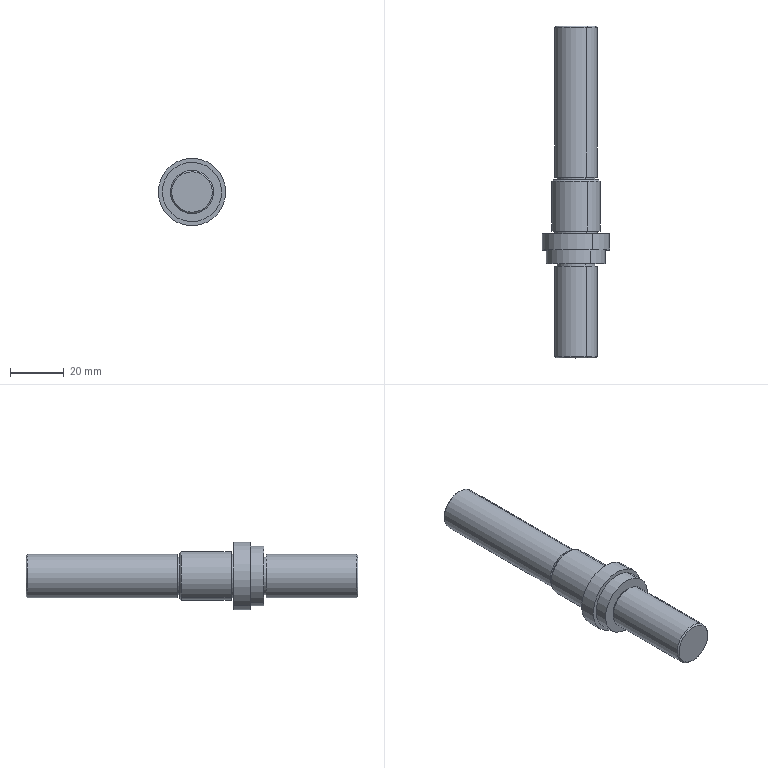Part | STEP file | 20304 | 1 solid | 31 faces | box 25 x 123 x 25 mm | volume 28266 mm3 | cylinder 16 | plane 9 | cone 6 | commonest cylinder face diameters 16 x6 14 x4 18 x2 22 x2 25 x2
STEP:
#1=CARTESIAN_POINT('',(3.356,-56.,6.143));
#2=VERTEX_POINT('',#1);
#3=CARTESIAN_POINT('',(-3.356,-56.,-6.143));
#4=VERTEX_POINT('',#3);
#5=CARTESIAN_POINT('',(0.,-56.,0.));
#6=DIRECTION('',(0.,1.,0.));
#7=AXIS2_PLACEMENT_3D('',#5,#6,$);
#8=CIRCLE('',#7,7.);
#9=EDGE_CURVE('',#2,#4,#8,.T.);
#10=ORIENTED_EDGE('',*,*,#9,.F.);
#11=CARTESIAN_POINT('',(3.356,-57.,6.143));
#12=VERTEX_POINT('',#11);
#13=CARTESIAN_POINT('',(3.356,-72.5,6.143));
#14=DIRECTION('',(0.,1.,0.));
#15=VECTOR('',#14,1.);
#16=LINE('',#13,#15);
#17=EDGE_CURVE('',#2,#12,#16,.F.);
#18=ORIENTED_EDGE('',*,*,#17,.T.);
#19=CARTESIAN_POINT('',(-3.356,-57.,-6.143));
#20=VERTEX_POINT('',#19);
#21=CARTESIAN_POINT('',(0.,-57.,0.));
#22=DIRECTION('',(0.,1.,0.));
#23=AXIS2_PLACEMENT_3D('',#21,#22,$);
#24=CIRCLE('',#23,7.);
#25=EDGE_CURVE('',#12,#20,#24,.T.);
#26=ORIENTED_EDGE('',*,*,#25,.T.);
#27=CARTESIAN_POINT('',(-3.356,-72.5,-6.143));
#28=DIRECTION('',(0.,1.,0.));
#29=VECTOR('',#28,1.);
#30=LINE('',#27,#29);
#31=EDGE_CURVE('',#4,#20,#30,.F.);
#32=ORIENTED_EDGE('',*,*,#31,.F.);
#33=EDGE_LOOP('',(#10,#18,#26,#32));
#34=FACE_OUTER_BOUND('',#33,.T.);
#35=CARTESIAN_POINT('',(0.,-61.5,0.));
#36=DIRECTION('',(0.,1.,0.));
#37=DIRECTION('',(0.4794,0.,0.8776));
#38=AXIS2_PLACEMENT_3D('',#35,#36,#37);
#39=CYLINDRICAL_SURFACE('',#38,7.);
#40=ADVANCED_FACE('',(#34),#39,.T.);
#41=CARTESIAN_POINT('',(0.,-56.,0.));
#42=DIRECTION('',(0.,1.,0.));
#43=AXIS2_PLACEMENT_3D('',#41,#42,$);
#44=CIRCLE('',#43,7.);
#45=EDGE_CURVE('',#4,#2,#44,.T.);
#46=ORIENTED_EDGE('',*,*,#45,.F.);
#47=ORIENTED_EDGE('',*,*,#31,.T.);
#48=CARTESIAN_POINT('',(0.,-57.,0.));
#49=DIRECTION('',(0.,1.,0.));
#50=AXIS2_PLACEMENT_3D('',#48,#49,$);
#51=CIRCLE('',#50,7.);
#52=EDGE_CURVE('',#20,#12,#51,.T.);
#53=ORIENTED_EDGE('',*,*,#52,.T.);
#54=ORIENTED_EDGE('',*,*,#17,.F.);
#55=EDGE_LOOP('',(#46,#47,#53,#54));
#56=FACE_OUTER_BOUND('',#55,.T.);
#57=ADVANCED_FACE('',(#56),#39,.T.);
#58=CARTESIAN_POINT('',(3.835,-76.,7.021));
#59=VERTEX_POINT('',#58);
#60=CARTESIAN_POINT('',(-3.835,-76.,-7.021));
#61=VERTEX_POINT('',#60);
#62=CARTESIAN_POINT('',(0.,-76.,0.));
#63=DIRECTION('',(0.,1.,0.));
#64=AXIS2_PLACEMENT_3D('',#62,#63,$);
#65=CIRCLE('',#64,8.);
#66=EDGE_CURVE('',#59,#61,#65,.T.);
#67=ORIENTED_EDGE('',*,*,#66,.F.);
#68=CARTESIAN_POINT('',(3.835,-77.,7.021));
#69=VERTEX_POINT('',#68);
#70=CARTESIAN_POINT('',(3.835,-61.5,7.021));
#71=DIRECTION('',(0.,1.,0.));
#72=VECTOR('',#71,1.);
#73=LINE('',#70,#72);
#74=EDGE_CURVE('',#59,#69,#73,.F.);
#75=ORIENTED_EDGE('',*,*,#74,.T.);
#76=CARTESIAN_POINT('',(-3.835,-77.,-7.021));
#77=VERTEX_POINT('',#76);
#78=CARTESIAN_POINT('',(0.,-77.,0.));
#79=DIRECTION('',(0.,1.,0.));
#80=AXIS2_PLACEMENT_3D('',#78,#79,$);
#81=CIRCLE('',#80,8.);
#82=EDGE_CURVE('',#69,#77,#81,.T.);
#83=ORIENTED_EDGE('',*,*,#82,.T.);
#84=CARTESIAN_POINT('',(-3.835,-61.5,-7.021));
#85=DIRECTION('',(0.,1.,0.));
#86=VECTOR('',#85,1.);
#87=LINE('',#84,#86);
#88=EDGE_CURVE('',#61,#77,#87,.F.);
#89=ORIENTED_EDGE('',*,*,#88,.F.);
#90=EDGE_LOOP('',(#67,#75,#83,#89));
#91=FACE_OUTER_BOUND('',#90,.T.);
#92=CARTESIAN_POINT('',(0.,-61.5,0.));
#93=DIRECTION('',(0.,1.,0.));
#94=DIRECTION('',(0.4794,0.,0.8776));
#95=AXIS2_PLACEMENT_3D('',#92,#93,#94);
#96=CYLINDRICAL_SURFACE('',#95,8.);
#97=ADVANCED_FACE('',(#91),#96,.T.);
#98=CARTESIAN_POINT('',(0.,-76.,0.));
#99=DIRECTION('',(0.,1.,0.));
#100=AXIS2_PLACEMENT_3D('',#98,#99,$);
#101=CIRCLE('',#100,8.);
#102=EDGE_CURVE('',#61,#59,#101,.T.);
#103=ORIENTED_EDGE('',*,*,#102,.F.);
#104=ORIENTED_EDGE('',*,*,#88,.T.);
#105=CARTESIAN_POINT('',(0.,-77.,0.));
#106=DIRECTION('',(0.,1.,0.));
#107=AXIS2_PLACEMENT_3D('',#105,#106,$);
#108=CIRCLE('',#107,8.);
#109=EDGE_CURVE('',#77,#69,#108,.T.);
#110=ORIENTED_EDGE('',*,*,#109,.T.);
#111=ORIENTED_EDGE('',*,*,#74,.F.);
#112=EDGE_LOOP('',(#103,#104,#110,#111));
#113=FACE_OUTER_BOUND('',#112,.T.);
#114=ADVANCED_FACE('',(#113),#96,.T.);
#115=CARTESIAN_POINT('',(5.993,-77.,10.97));
#116=VERTEX_POINT('',#115);
#117=CARTESIAN_POINT('',(-5.993,-77.,-10.97));
#118=VERTEX_POINT('',#117);
#119=CARTESIAN_POINT('',(0.,-77.,0.));
#120=DIRECTION('',(0.,1.,0.));
#121=AXIS2_PLACEMENT_3D('',#119,#120,$);
#122=CIRCLE('',#121,12.5);
#123=EDGE_CURVE('',#116,#118,#122,.T.);
#124=ORIENTED_EDGE('',*,*,#123,.F.);
#125=CARTESIAN_POINT('',(5.993,-83.,10.97));
#126=VERTEX_POINT('',#125);
#127=CARTESIAN_POINT('',(5.993,-80.,10.97));
#128=DIRECTION('',(0.,1.,0.));
#129=VECTOR('',#128,1.);
#130=LINE('',#127,#129);
#131=EDGE_CURVE('',#116,#126,#130,.F.);
#132=ORIENTED_EDGE('',*,*,#131,.T.);
#133=CARTESIAN_POINT('',(-5.993,-83.,-10.97));
#134=VERTEX_POINT('',#133);
#135=CARTESIAN_POINT('',(0.,-83.,0.));
#136=DIRECTION('',(0.,1.,0.));
#137=AXIS2_PLACEMENT_3D('',#135,#136,$);
#138=CIRCLE('',#137,12.5);
#139=EDGE_CURVE('',#126,#134,#138,.T.);
#140=ORIENTED_EDGE('',*,*,#139,.T.);
#141=CARTESIAN_POINT('',(-5.993,-80.,-10.97));
#142=DIRECTION('',(0.,1.,0.));
#143=VECTOR('',#142,1.);
#144=LINE('',#141,#143);
#145=EDGE_CURVE('',#118,#134,#144,.F.);
#146=ORIENTED_EDGE('',*,*,#145,.F.);
#147=EDGE_LOOP('',(#124,#132,#140,#146));
#148=FACE_OUTER_BOUND('',#147,.T.);
#149=CARTESIAN_POINT('',(0.,-61.5,0.));
#150=DIRECTION('',(0.,1.,0.));
#151=DIRECTION('',(0.4794,0.,0.8776));
#152=AXIS2_PLACEMENT_3D('',#149,#150,#151);
#153=CYLINDRICAL_SURFACE('',#152,12.5);
#154=ADVANCED_FACE('',(#148),#153,.T.);
#155=CARTESIAN_POINT('',(0.,-77.,0.));
#156=DIRECTION('',(0.,1.,0.));
#157=AXIS2_PLACEMENT_3D('',#155,#156,$);
#158=CIRCLE('',#157,12.5);
#159=EDGE_CURVE('',#118,#116,#158,.T.);
#160=ORIENTED_EDGE('',*,*,#159,.F.);
#161=ORIENTED_EDGE('',*,*,#145,.T.);
#162=CARTESIAN_POINT('',(0.,-83.,0.));
#163=DIRECTION('',(0.,1.,0.));
#164=AXIS2_PLACEMENT_3D('',#162,#163,$);
#165=CIRCLE('',#164,12.5);
#166=EDGE_CURVE('',#134,#126,#165,.T.);
#167=ORIENTED_EDGE('',*,*,#166,.T.);
#168=ORIENTED_EDGE('',*,*,#131,.F.);
#169=EDGE_LOOP('',(#160,#161,#167,#168));
#170=FACE_OUTER_BOUND('',#169,.T.);
#171=ADVANCED_FACE('',(#170),#153,.T.);
#172=CARTESIAN_POINT('',(5.274,-83.,9.653));
#173=VERTEX_POINT('',#172);
#174=CARTESIAN_POINT('',(-5.274,-83.,-9.653));
#175=VERTEX_POINT('',#174);
#176=CARTESIAN_POINT('',(0.,-83.,0.));
#177=DIRECTION('',(0.,1.,0.));
#178=AXIS2_PLACEMENT_3D('',#176,#177,$);
#179=CIRCLE('',#178,11.);
#180=EDGE_CURVE('',#173,#175,#179,.T.);
#181=ORIENTED_EDGE('',*,*,#180,.F.);
#182=CARTESIAN_POINT('',(5.274,-88.,9.653));
#183=VERTEX_POINT('',#182);
#184=CARTESIAN_POINT('',(5.274,-85.5,9.653));
#185=DIRECTION('',(0.,1.,0.));
#186=VECTOR('',#185,1.);
#187=LINE('',#184,#186);
#188=EDGE_CURVE('',#173,#183,#187,.F.);
#189=ORIENTED_EDGE('',*,*,#188,.T.);
#190=CARTESIAN_POINT('',(-5.274,-88.,-9.653));
#191=VERTEX_POINT('',#190);
#192=CARTESIAN_POINT('',(0.,-88.,0.));
#193=DIRECTION('',(0.,1.,0.));
#194=AXIS2_PLACEMENT_3D('',#192,#193,$);
#195=CIRCLE('',#194,11.);
#196=EDGE_CURVE('',#183,#191,#195,.T.);
#197=ORIENTED_EDGE('',*,*,#196,.T.);
#198=CARTESIAN_POINT('',(-5.274,-85.5,-9.653));
#199=DIRECTION('',(0.,1.,0.));
#200=VECTOR('',#199,1.);
#201=LINE('',#198,#200);
#202=EDGE_CURVE('',#175,#191,#201,.F.);
#203=ORIENTED_EDGE('',*,*,#202,.F.);
#204=EDGE_LOOP('',(#181,#189,#197,#203));
#205=FACE_OUTER_BOUND('',#204,.T.);
#206=CARTESIAN_POINT('',(0.,-61.5,0.));
#207=DIRECTION('',(0.,1.,0.));
#208=DIRECTION('',(0.4794,0.,0.8776));
#209=AXIS2_PLACEMENT_3D('',#206,#207,#208);
#210=CYLINDRICAL_SURFACE('',#209,11.);
#211=ADVANCED_FACE('',(#205),#210,.T.);
#212=CARTESIAN_POINT('',(0.,-83.,0.));
#213=DIRECTION('',(0.,1.,0.));
#214=AXIS2_PLACEMENT_3D('',#212,#213,$);
#215=CIRCLE('',#214,11.);
#216=EDGE_CURVE('',#175,#173,#215,.T.);
#217=ORIENTED_EDGE('',*,*,#216,.F.);
#218=ORIENTED_EDGE('',*,*,#202,.T.);
#219=CARTESIAN_POINT('',(0.,-88.,0.));
#220=DIRECTION('',(0.,1.,0.));
#221=AXIS2_PLACEMENT_3D('',#219,#220,$);
#222=CIRCLE('',#221,11.);
#223=EDGE_CURVE('',#191,#183,#222,.T.);
#224=ORIENTED_EDGE('',*,*,#223,.T.);
#225=ORIENTED_EDGE('',*,*,#188,.F.);
#226=EDGE_LOOP('',(#217,#218,#224,#225));
#227=FACE_OUTER_BOUND('',#226,.T.);
#228=ADVANCED_FACE('',(#227),#210,.T.);
#229=CARTESIAN_POINT('',(3.356,-88.,6.143));
#230=VERTEX_POINT('',#229);
#231=CARTESIAN_POINT('',(-3.356,-88.,-6.143));
#232=VERTEX_POINT('',#231);
#233=CARTESIAN_POINT('',(0.,-88.,0.));
#234=DIRECTION('',(0.,1.,0.));
#235=AXIS2_PLACEMENT_3D('',#233,#234,$);
#236=CIRCLE('',#235,7.);
#237=EDGE_CURVE('',#230,#232,#236,.T.);
#238=ORIENTED_EDGE('',*,*,#237,.F.);
#239=CARTESIAN_POINT('',(3.356,-89.,6.143));
#240=VERTEX_POINT('',#239);
#241=CARTESIAN_POINT('',(3.356,-72.5,6.143));
#242=DIRECTION('',(0.,1.,0.));
#243=VECTOR('',#242,1.);
#244=LINE('',#241,#243);
#245=EDGE_CURVE('',#230,#240,#244,.F.);
#246=ORIENTED_EDGE('',*,*,#245,.T.);
#247=CARTESIAN_POINT('',(-3.356,-89.,-6.143));
#248=VERTEX_POINT('',#247);
#249=CARTESIAN_POINT('',(0.,-89.,0.));
#250=DIRECTION('',(0.,1.,0.));
#251=AXIS2_PLACEMENT_3D('',#249,#250,$);
#252=CIRCLE('',#251,7.);
#253=EDGE_CURVE('',#240,#248,#252,.T.);
#254=ORIENTED_EDGE('',*,*,#253,.T.);
#255=CARTESIAN_POINT('',(-3.356,-72.5,-6.143));
#256=DIRECTION('',(0.,1.,0.));
#257=VECTOR('',#256,1.);
#258=LINE('',#255,#257);
#259=EDGE_CURVE('',#232,#248,#258,.F.);
#260=ORIENTED_EDGE('',*,*,#259,.F.);
#261=EDGE_LOOP('',(#238,#246,#254,#260));
#262=FACE_OUTER_BOUND('',#261,.T.);
#263=ADVANCED_FACE('',(#262),#39,.T.);
#264=CARTESIAN_POINT('',(0.,-88.,0.));
#265=DIRECTION('',(0.,1.,0.));
#266=AXIS2_PLACEMENT_3D('',#264,#265,$);
#267=CIRCLE('',#266,7.);
#268=EDGE_CURVE('',#232,#230,#267,.T.);
#269=ORIENTED_EDGE('',*,*,#268,.F.);
#270=ORIENTED_EDGE('',*,*,#259,.T.);
#271=CARTESIAN_POINT('',(0.,-89.,0.));
#272=DIRECTION('',(0.,1.,0.));
#273=AXIS2_PLACEMENT_3D('',#271,#272,$);
#274=CIRCLE('',#273,7.);
#275=EDGE_CURVE('',#248,#240,#274,.T.);
#276=ORIENTED_EDGE('',*,*,#275,.T.);
#277=ORIENTED_EDGE('',*,*,#245,.F.);
#278=EDGE_LOOP('',(#269,#270,#276,#277));
#279=FACE_OUTER_BOUND('',#278,.T.);
#280=ADVANCED_FACE('',(#279),#39,.T.);
#281=CARTESIAN_POINT('',(3.835,-56.,7.021));
#282=VERTEX_POINT('',#281);
#283=CARTESIAN_POINT('',(-3.835,-56.,-7.021));
#284=VERTEX_POINT('',#283);
#285=CARTESIAN_POINT('',(0.,-56.,0.));
#286=DIRECTION('',(0.,1.,0.));
#287=AXIS2_PLACEMENT_3D('',#285,#286,$);
#288=CIRCLE('',#287,8.);
#289=EDGE_CURVE('',#282,#284,#288,.T.);
#290=ORIENTED_EDGE('',*,*,#289,.F.);
#291=CARTESIAN_POINT('',(0.,-56.,0.));
#292=DIRECTION('',(0.,1.,0.));
#293=AXIS2_PLACEMENT_3D('',#291,#292,$);
#294=CIRCLE('',#293,8.);
#295=EDGE_CURVE('',#284,#282,#294,.T.);
#296=ORIENTED_EDGE('',*,*,#295,.F.);
#297=EDGE_LOOP('',(#290,#296));
#298=FACE_OUTER_BOUND('',#297,.T.);
#299=ORIENTED_EDGE('',*,*,#45,.T.);
#300=ORIENTED_EDGE('',*,*,#9,.T.);
#301=EDGE_LOOP('',(#299,#300));
#302=FACE_BOUND('',#301,.T.);
#303=CARTESIAN_POINT('',(0.,-56.,8.));
#304=DIRECTION('',(0.,1.,0.));
#305=DIRECTION('',(1.,0.,0.));
#306=AXIS2_PLACEMENT_3D('',#303,#304,#305);
#307=PLANE('',#306);
#308=ADVANCED_FACE('',(#298,#302),#307,.F.);
#309=CARTESIAN_POINT('',(4.315,-76.,7.898));
#310=VERTEX_POINT('',#309);
#311=CARTESIAN_POINT('',(-4.315,-76.,-7.898));
#312=VERTEX_POINT('',#311);
#313=CARTESIAN_POINT('',(0.,-76.,0.));
#314=DIRECTION('',(0.,1.,0.));
#315=AXIS2_PLACEMENT_3D('',#313,#314,$);
#316=CIRCLE('',#315,9.);
#317=EDGE_CURVE('',#310,#312,#316,.T.);
#318=ORIENTED_EDGE('',*,*,#317,.F.);
#319=CARTESIAN_POINT('',(0.,-76.,0.));
#320=DIRECTION('',(0.,1.,0.));
#321=AXIS2_PLACEMENT_3D('',#319,#320,$);
#322=CIRCLE('',#321,9.);
#323=EDGE_CURVE('',#312,#310,#322,.T.);
#324=ORIENTED_EDGE('',*,*,#323,.F.);
#325=EDGE_LOOP('',(#318,#324));
#326=FACE_OUTER_BOUND('',#325,.T.);
#327=ORIENTED_EDGE('',*,*,#102,.T.);
#328=ORIENTED_EDGE('',*,*,#66,.T.);
#329=EDGE_LOOP('',(#327,#328));
#330=FACE_BOUND('',#329,.T.);
#331=CARTESIAN_POINT('',(0.,-76.,9.));
#332=DIRECTION('',(0.,1.,0.));
#333=DIRECTION('',(1.,0.,0.));
#334=AXIS2_PLACEMENT_3D('',#331,#332,#333);
#335=PLANE('',#334);
#336=ADVANCED_FACE('',(#326,#330),#335,.F.);
#337=ORIENTED_EDGE('',*,*,#159,.T.);
#338=ORIENTED_EDGE('',*,*,#123,.T.);
#339=EDGE_LOOP('',(#337,#338));
#340=FACE_OUTER_BOUND('',#339,.T.);
#341=ORIENTED_EDGE('',*,*,#82,.F.);
#342=ORIENTED_EDGE('',*,*,#109,.F.);
#343=EDGE_LOOP('',(#341,#342));
#344=FACE_BOUND('',#343,.T.);
#345=CARTESIAN_POINT('',(0.,-77.,8.));
#346=DIRECTION('',(0.,1.,0.));
#347=DIRECTION('',(1.,0.,0.));
#348=AXIS2_PLACEMENT_3D('',#345,#346,#347);
#349=PLANE('',#348);
#350=ADVANCED_FACE('',(#340,#344),#349,.T.);
#351=ORIENTED_EDGE('',*,*,#139,.F.);
#352=ORIENTED_EDGE('',*,*,#166,.F.);
#353=EDGE_LOOP('',(#351,#352));
#354=FACE_OUTER_BOUND('',#353,.T.);
#355=ORIENTED_EDGE('',*,*,#216,.T.);
#356=ORIENTED_EDGE('',*,*,#180,.T.);
#357=EDGE_LOOP('',(#355,#356));
#358=FACE_BOUND('',#357,.T.);
#359=CARTESIAN_POINT('',(0.,-83.,12.5));
#360=DIRECTION('',(0.,1.,0.));
#361=DIRECTION('',(1.,0.,0.));
#362=AXIS2_PLACEMENT_3D('',#359,#360,#361);
#363=PLANE('',#362);
#364=ADVANCED_FACE('',(#354,#358),#363,.F.);
#365=ORIENTED_EDGE('',*,*,#196,.F.);
#366=ORIENTED_EDGE('',*,*,#223,.F.);
#367=EDGE_LOOP('',(#365,#366));
#368=FACE_OUTER_BOUND('',#367,.T.);
#369=ORIENTED_EDGE('',*,*,#268,.T.);
#370=ORIENTED_EDGE('',*,*,#237,.T.);
#371=EDGE_LOOP('',(#369,#370));
#372=FACE_BOUND('',#371,.T.);
#373=CARTESIAN_POINT('',(0.,-88.,11.));
#374=DIRECTION('',(0.,1.,0.));
#375=DIRECTION('',(1.,0.,0.));
#376=AXIS2_PLACEMENT_3D('',#373,#374,#375);
#377=PLANE('',#376);
#378=ADVANCED_FACE('',(#368,#372),#377,.F.);
#379=CARTESIAN_POINT('',(-3.835,-89.,-7.021));
#380=VERTEX_POINT('',#379);
#381=CARTESIAN_POINT('',(3.835,-89.,7.021));
#382=VERTEX_POINT('',#381);
#383=CARTESIAN_POINT('',(0.,-89.,0.));
#384=DIRECTION('',(0.,1.,0.));
#385=AXIS2_PLACEMENT_3D('',#383,#384,$);
#386=CIRCLE('',#385,8.);
#387=EDGE_CURVE('',#380,#382,#386,.T.);
#388=ORIENTED_EDGE('',*,*,#387,.T.);
#389=CARTESIAN_POINT('',(0.,-89.,0.));
#390=DIRECTION('',(0.,1.,0.));
#391=AXIS2_PLACEMENT_3D('',#389,#390,$);
#392=CIRCLE('',#391,8.);
#393=EDGE_CURVE('',#382,#380,#392,.T.);
#394=ORIENTED_EDGE('',*,*,#393,.T.);
#395=EDGE_LOOP('',(#388,#394));
#396=FACE_OUTER_BOUND('',#395,.T.);
#397=ORIENTED_EDGE('',*,*,#253,.F.);
#398=ORIENTED_EDGE('',*,*,#275,.F.);
#399=EDGE_LOOP('',(#397,#398));
#400=FACE_BOUND('',#399,.T.);
#401=CARTESIAN_POINT('',(0.,-89.,7.));
#402=DIRECTION('',(0.,1.,0.));
#403=DIRECTION('',(1.,0.,0.));
#404=AXIS2_PLACEMENT_3D('',#401,#402,#403);
#405=PLANE('',#404);
#406=ADVANCED_FACE('',(#396,#400),#405,.T.);
#407=CARTESIAN_POINT('',(3.835,-0.5,7.021));
#408=VERTEX_POINT('',#407);
#409=CARTESIAN_POINT('',(3.835,-61.5,7.021));
#410=DIRECTION('',(0.,1.,0.));
#411=VECTOR('',#410,1.);
#412=LINE('',#409,#411);
#413=EDGE_CURVE('',#408,#282,#412,.F.);
#414=ORIENTED_EDGE('',*,*,#413,.T.);
#415=ORIENTED_EDGE('',*,*,#289,.T.);
#416=CARTESIAN_POINT('',(-3.835,-0.5,-7.021));
#417=VERTEX_POINT('',#416);
#418=CARTESIAN_POINT('',(-3.835,-61.5,-7.021));
#419=DIRECTION('',(0.,1.,0.));
#420=VECTOR('',#419,1.);
#421=LINE('',#418,#420);
#422=EDGE_CURVE('',#417,#284,#421,.F.);
#423=ORIENTED_EDGE('',*,*,#422,.F.);
#424=CARTESIAN_POINT('',(0.,-0.5,0.));
#425=DIRECTION('',(0.,1.,0.));
#426=AXIS2_PLACEMENT_3D('',#424,#425,$);
#427=CIRCLE('',#426,8.);
#428=EDGE_CURVE('',#408,#417,#427,.T.);
#429=ORIENTED_EDGE('',*,*,#428,.F.);
#430=EDGE_LOOP('',(#414,#415,#423,#429));
#431=FACE_OUTER_BOUND('',#430,.T.);
#432=ADVANCED_FACE('',(#431),#96,.T.);
#433=ORIENTED_EDGE('',*,*,#422,.T.);
#434=ORIENTED_EDGE('',*,*,#295,.T.);
#435=ORIENTED_EDGE('',*,*,#413,.F.);
#436=CARTESIAN_POINT('',(0.,-0.5,0.));
#437=DIRECTION('',(0.,1.,0.));
#438=AXIS2_PLACEMENT_3D('',#436,#437,$);
#439=CIRCLE('',#438,8.);
#440=EDGE_CURVE('',#417,#408,#439,.T.);
#441=ORIENTED_EDGE('',*,*,#440,.F.);
#442=EDGE_LOOP('',(#433,#434,#435,#441));
#443=FACE_OUTER_BOUND('',#442,.T.);
#444=ADVANCED_FACE('',(#443),#96,.T.);
#445=CARTESIAN_POINT('',(3.596,0.,6.582));
#446=VERTEX_POINT('',#445);
#447=CARTESIAN_POINT('',(-3.596,0.,-6.582));
#448=VERTEX_POINT('',#447);
#449=CARTESIAN_POINT('',(0.,0.,0.));
#450=DIRECTION('',(0.,1.,0.));
#451=AXIS2_PLACEMENT_3D('',#449,#450,$);
#452=CIRCLE('',#451,7.5);
#453=EDGE_CURVE('',#446,#448,#452,.T.);
#454=ORIENTED_EDGE('',*,*,#453,.T.);
#455=CARTESIAN_POINT('',(0.,0.,0.));
#456=DIRECTION('',(0.,1.,0.));
#457=AXIS2_PLACEMENT_3D('',#455,#456,$);
#458=CIRCLE('',#457,7.5);
#459=EDGE_CURVE('',#448,#446,#458,.T.);
#460=ORIENTED_EDGE('',*,*,#459,.T.);
#461=EDGE_LOOP('',(#454,#460));
#462=FACE_OUTER_BOUND('',#461,.T.);
#463=CARTESIAN_POINT('',(0.,0.,0.));
#464=DIRECTION('',(0.,1.,0.));
#465=DIRECTION('',(1.,0.,0.));
#466=AXIS2_PLACEMENT_3D('',#463,#464,#465);
#467=PLANE('',#466);
#468=ADVANCED_FACE('',(#462),#467,.T.);
#469=CARTESIAN_POINT('',(3.716,-0.25,6.801));
#470=DIRECTION('',(0.339,-0.7071,0.6205));
#471=VECTOR('',#470,1.);
#472=LINE('',#469,#471);
#473=EDGE_CURVE('',#446,#408,#472,.T.);
#474=ORIENTED_EDGE('',*,*,#473,.T.);
#475=ORIENTED_EDGE('',*,*,#428,.T.);
#476=CARTESIAN_POINT('',(-3.716,-0.25,-6.801));
#477=DIRECTION('',(-0.339,-0.7071,-0.6205));
#478=VECTOR('',#477,1.);
#479=LINE('',#476,#478);
#480=EDGE_CURVE('',#448,#417,#479,.T.);
#481=ORIENTED_EDGE('',*,*,#480,.F.);
#482=ORIENTED_EDGE('',*,*,#453,.F.);
#483=EDGE_LOOP('',(#474,#475,#481,#482));
#484=FACE_OUTER_BOUND('',#483,.T.);
#485=CARTESIAN_POINT('',(0.,7.5,0.));
#486=DIRECTION('',(0.,-1.,0.));
#487=DIRECTION('',(0.4794,0.,0.8776));
#488=AXIS2_PLACEMENT_3D('',#485,#486,#487);
#489=CONICAL_SURFACE('',#488,0.,0.7854);
#490=ADVANCED_FACE('',(#484),#489,.T.);
#491=ORIENTED_EDGE('',*,*,#480,.T.);
#492=ORIENTED_EDGE('',*,*,#440,.T.);
#493=ORIENTED_EDGE('',*,*,#473,.F.);
#494=ORIENTED_EDGE('',*,*,#459,.F.);
#495=EDGE_LOOP('',(#491,#492,#493,#494));
#496=FACE_OUTER_BOUND('',#495,.T.);
#497=CARTESIAN_POINT('',(0.,7.5,0.));
#498=DIRECTION('',(0.,-1.,0.));
#499=DIRECTION('',(0.008915,0.,-1.));
#500=AXIS2_PLACEMENT_3D('',#497,#498,#499);
#501=CONICAL_SURFACE('',#500,0.,0.7854);
#502=ADVANCED_FACE('',(#496),#501,.T.);
#503=CARTESIAN_POINT('',(4.315,-57.5,7.898));
#504=VERTEX_POINT('',#503);
#505=CARTESIAN_POINT('',(4.315,-66.5,7.898));
#506=DIRECTION('',(0.,1.,0.));
#507=VECTOR('',#506,1.);
#508=LINE('',#505,#507);
#509=EDGE_CURVE('',#504,#310,#508,.F.);
#510=ORIENTED_EDGE('',*,*,#509,.T.);
#511=ORIENTED_EDGE('',*,*,#317,.T.);
#512=CARTESIAN_POINT('',(-4.315,-57.5,-7.898));
#513=VERTEX_POINT('',#512);
#514=CARTESIAN_POINT('',(-4.315,-66.5,-7.898));
#515=DIRECTION('',(0.,1.,0.));
#516=VECTOR('',#515,1.);
#517=LINE('',#514,#516);
#518=EDGE_CURVE('',#513,#312,#517,.F.);
#519=ORIENTED_EDGE('',*,*,#518,.F.);
#520=CARTESIAN_POINT('',(0.,-57.5,0.));
#521=DIRECTION('',(0.,1.,0.));
#522=AXIS2_PLACEMENT_3D('',#520,#521,$);
#523=CIRCLE('',#522,9.);
#524=EDGE_CURVE('',#504,#513,#523,.T.);
#525=ORIENTED_EDGE('',*,*,#524,.F.);
#526=EDGE_LOOP('',(#510,#511,#519,#525));
#527=FACE_OUTER_BOUND('',#526,.T.);
#528=CARTESIAN_POINT('',(0.,-61.5,0.));
#529=DIRECTION('',(0.,1.,0.));
#530=DIRECTION('',(0.4794,0.,0.8776));
#531=AXIS2_PLACEMENT_3D('',#528,#529,#530);
#532=CYLINDRICAL_SURFACE('',#531,9.);
#533=ADVANCED_FACE('',(#527),#532,.T.);
#534=ORIENTED_EDGE('',*,*,#518,.T.);
#535=ORIENTED_EDGE('',*,*,#323,.T.);
#536=ORIENTED_EDGE('',*,*,#509,.F.);
#537=CARTESIAN_POINT('',(0.,-57.5,0.));
#538=DIRECTION('',(0.,1.,0.));
#539=AXIS2_PLACEMENT_3D('',#537,#538,$);
#540=CIRCLE('',#539,9.);
#541=EDGE_CURVE('',#513,#504,#540,.T.);
#542=ORIENTED_EDGE('',*,*,#541,.F.);
#543=EDGE_LOOP('',(#534,#535,#536,#542));
#544=FACE_OUTER_BOUND('',#543,.T.);
#545=ADVANCED_FACE('',(#544),#532,.T.);
#546=CARTESIAN_POINT('',(4.075,-57.,7.459));
#547=VERTEX_POINT('',#546);
#548=CARTESIAN_POINT('',(-4.075,-57.,-7.459));
#549=VERTEX_POINT('',#548);
#550=CARTESIAN_POINT('',(0.,-57.,0.));
#551=DIRECTION('',(0.,1.,0.));
#552=AXIS2_PLACEMENT_3D('',#550,#551,$);
#553=CIRCLE('',#552,8.5);
#554=EDGE_CURVE('',#547,#549,#553,.T.);
#555=ORIENTED_EDGE('',*,*,#554,.T.);
#556=CARTESIAN_POINT('',(0.,-57.,0.));
#557=DIRECTION('',(0.,1.,0.));
#558=AXIS2_PLACEMENT_3D('',#556,#557,$);
#559=CIRCLE('',#558,8.5);
#560=EDGE_CURVE('',#549,#547,#559,.T.);
#561=ORIENTED_EDGE('',*,*,#560,.T.);
#562=EDGE_LOOP('',(#555,#561));
#563=FACE_OUTER_BOUND('',#562,.T.);
#564=ORIENTED_EDGE('',*,*,#25,.F.);
#565=ORIENTED_EDGE('',*,*,#52,.F.);
#566=EDGE_LOOP('',(#564,#565));
#567=FACE_BOUND('',#566,.T.);
#568=CARTESIAN_POINT('',(0.,-57.,7.));
#569=DIRECTION('',(0.,1.,0.));
#570=DIRECTION('',(1.,0.,0.));
#571=AXIS2_PLACEMENT_3D('',#568,#569,#570);
#572=PLANE('',#571);
#573=ADVANCED_FACE('',(#563,#567),#572,.T.);
#574=CARTESIAN_POINT('',(4.195,-57.25,7.679));
#575=DIRECTION('',(0.339,-0.7071,0.6205));
#576=VECTOR('',#575,1.);
#577=LINE('',#574,#576);
#578=EDGE_CURVE('',#547,#504,#577,.T.);
#579=ORIENTED_EDGE('',*,*,#578,.T.);
#580=ORIENTED_EDGE('',*,*,#524,.T.);
#581=CARTESIAN_POINT('',(-4.195,-57.25,-7.679));
#582=DIRECTION('',(-0.339,-0.7071,-0.6205));
#583=VECTOR('',#582,1.);
#584=LINE('',#581,#583);
#585=EDGE_CURVE('',#549,#513,#584,.T.);
#586=ORIENTED_EDGE('',*,*,#585,.F.);
#587=ORIENTED_EDGE('',*,*,#554,.F.);
#588=EDGE_LOOP('',(#579,#580,#586,#587));
#589=FACE_OUTER_BOUND('',#588,.T.);
#590=CARTESIAN_POINT('',(0.,-48.5,0.));
#591=DIRECTION('',(0.,-1.,0.));
#592=DIRECTION('',(0.4794,0.,0.8776));
#593=AXIS2_PLACEMENT_3D('',#590,#591,#592);
#594=CONICAL_SURFACE('',#593,0.,0.7854);
#595=ADVANCED_FACE('',(#589),#594,.T.);
#596=ORIENTED_EDGE('',*,*,#585,.T.);
#597=ORIENTED_EDGE('',*,*,#541,.T.);
#598=ORIENTED_EDGE('',*,*,#578,.F.);
#599=ORIENTED_EDGE('',*,*,#560,.F.);
#600=EDGE_LOOP('',(#596,#597,#598,#599));
#601=FACE_OUTER_BOUND('',#600,.T.);
#602=CARTESIAN_POINT('',(0.,-48.5,0.));
#603=DIRECTION('',(0.,-1.,0.));
#604=DIRECTION('',(-0.02227,0.,-0.9998));
#605=AXIS2_PLACEMENT_3D('',#602,#603,#604);
#606=CONICAL_SURFACE('',#605,0.,0.7854);
#607=ADVANCED_FACE('',(#601),#606,.T.);
#608=CARTESIAN_POINT('',(-3.835,-122.5,-7.021));
#609=VERTEX_POINT('',#608);
#610=CARTESIAN_POINT('',(-3.835,-61.5,-7.021));
#611=DIRECTION('',(0.,1.,0.));
#612=VECTOR('',#611,1.);
#613=LINE('',#610,#612);
#614=EDGE_CURVE('',#380,#609,#613,.F.);
#615=ORIENTED_EDGE('',*,*,#614,.F.);
#616=ORIENTED_EDGE('',*,*,#393,.F.);
#617=CARTESIAN_POINT('',(3.835,-122.5,7.021));
#618=VERTEX_POINT('',#617);
#619=CARTESIAN_POINT('',(3.835,-61.5,7.021));
#620=DIRECTION('',(0.,1.,0.));
#621=VECTOR('',#620,1.);
#622=LINE('',#619,#621);
#623=EDGE_CURVE('',#382,#618,#622,.F.);
#624=ORIENTED_EDGE('',*,*,#623,.T.);
#625=CARTESIAN_POINT('',(0.,-122.5,0.));
#626=DIRECTION('',(0.,1.,0.));
#627=AXIS2_PLACEMENT_3D('',#625,#626,$);
#628=CIRCLE('',#627,8.);
#629=EDGE_CURVE('',#618,#609,#628,.T.);
#630=ORIENTED_EDGE('',*,*,#629,.T.);
#631=EDGE_LOOP('',(#615,#616,#624,#630));
#632=FACE_OUTER_BOUND('',#631,.T.);
#633=ADVANCED_FACE('',(#632),#96,.T.);
#634=ORIENTED_EDGE('',*,*,#623,.F.);
#635=ORIENTED_EDGE('',*,*,#387,.F.);
#636=ORIENTED_EDGE('',*,*,#614,.T.);
#637=CARTESIAN_POINT('',(0.,-122.5,0.));
#638=DIRECTION('',(0.,1.,0.));
#639=AXIS2_PLACEMENT_3D('',#637,#638,$);
#640=CIRCLE('',#639,8.);
#641=EDGE_CURVE('',#609,#618,#640,.T.);
#642=ORIENTED_EDGE('',*,*,#641,.T.);
#643=EDGE_LOOP('',(#634,#635,#636,#642));
#644=FACE_OUTER_BOUND('',#643,.T.);
#645=ADVANCED_FACE('',(#644),#96,.T.);
#646=CARTESIAN_POINT('',(-3.596,-123.,-6.582));
#647=VERTEX_POINT('',#646);
#648=CARTESIAN_POINT('',(3.596,-123.,6.582));
#649=VERTEX_POINT('',#648);
#650=CARTESIAN_POINT('',(0.,-123.,0.));
#651=DIRECTION('',(0.,1.,0.));
#652=AXIS2_PLACEMENT_3D('',#650,#651,$);
#653=CIRCLE('',#652,7.5);
#654=EDGE_CURVE('',#647,#649,#653,.T.);
#655=ORIENTED_EDGE('',*,*,#654,.F.);
#656=CARTESIAN_POINT('',(0.,-123.,0.));
#657=DIRECTION('',(0.,1.,0.));
#658=AXIS2_PLACEMENT_3D('',#656,#657,$);
#659=CIRCLE('',#658,7.5);
#660=EDGE_CURVE('',#649,#647,#659,.T.);
#661=ORIENTED_EDGE('',*,*,#660,.F.);
#662=EDGE_LOOP('',(#655,#661));
#663=FACE_OUTER_BOUND('',#662,.T.);
#664=CARTESIAN_POINT('',(0.,-123.,8.));
#665=DIRECTION('',(0.,1.,0.));
#666=DIRECTION('',(1.,0.,0.));
#667=AXIS2_PLACEMENT_3D('',#664,#665,#666);
#668=PLANE('',#667);
#669=ADVANCED_FACE('',(#663),#668,.F.);
#670=CARTESIAN_POINT('',(3.716,-122.75,6.801));
#671=DIRECTION('',(0.339,0.7071,0.6205));
#672=VECTOR('',#671,1.);
#673=LINE('',#670,#672);
#674=EDGE_CURVE('',#618,#649,#673,.F.);
#675=ORIENTED_EDGE('',*,*,#674,.T.);
#676=ORIENTED_EDGE('',*,*,#660,.T.);
#677=CARTESIAN_POINT('',(-3.716,-122.75,-6.801));
#678=DIRECTION('',(-0.339,0.7071,-0.6205));
#679=VECTOR('',#678,1.);
#680=LINE('',#677,#679);
#681=EDGE_CURVE('',#609,#647,#680,.F.);
#682=ORIENTED_EDGE('',*,*,#681,.F.);
#683=ORIENTED_EDGE('',*,*,#629,.F.);
#684=EDGE_LOOP('',(#675,#676,#682,#683));
#685=FACE_OUTER_BOUND('',#684,.T.);
#686=CARTESIAN_POINT('',(0.,-130.5,0.));
#687=DIRECTION('',(0.,1.,0.));
#688=DIRECTION('',(0.4794,0.,0.8776));
#689=AXIS2_PLACEMENT_3D('',#686,#687,#688);
#690=CONICAL_SURFACE('',#689,0.,0.7854);
#691=ADVANCED_FACE('',(#685),#690,.T.);
#692=ORIENTED_EDGE('',*,*,#681,.T.);
#693=ORIENTED_EDGE('',*,*,#654,.T.);
#694=ORIENTED_EDGE('',*,*,#674,.F.);
#695=ORIENTED_EDGE('',*,*,#641,.F.);
#696=EDGE_LOOP('',(#692,#693,#694,#695));
#697=FACE_OUTER_BOUND('',#696,.T.);
#698=CARTESIAN_POINT('',(0.,-130.5,0.));
#699=DIRECTION('',(0.,1.,0.));
#700=DIRECTION('',(0.128,0.,-0.9918));
#701=AXIS2_PLACEMENT_3D('',#698,#699,#700);
#702=CONICAL_SURFACE('',#701,0.,0.7854);
#703=ADVANCED_FACE('',(#697),#702,.T.);
#704=CLOSED_SHELL('',(#40,#57,#97,#114,#154,#171,#211,#228,#263,#280,#308,#336,#350,#364,#378,#406,#432,#444,#468,#490,#502,#533,#545,#573,#595,#607,#633,#645,#669,#691,#703));
#705=MANIFOLD_SOLID_BREP('',#704);
#706=(LENGTH_UNIT()NAMED_UNIT(*)SI_UNIT(.MILLI.,.METRE.));
#707=UNCERTAINTY_MEASURE_WITH_UNIT(LENGTH_MEASURE(0.005),#706,'','');
#708=(NAMED_UNIT(*)PLANE_ANGLE_UNIT()SI_UNIT($,.RADIAN.));
#709=(NAMED_UNIT(*)SI_UNIT($,.STERADIAN.)SOLID_ANGLE_UNIT());
#710=(GEOMETRIC_REPRESENTATION_CONTEXT(3)GLOBAL_UNCERTAINTY_ASSIGNED_CONTEXT((#707))GLOBAL_UNIT_ASSIGNED_CONTEXT((#706,#708,#709))REPRESENTATION_CONTEXT('',''));
#711=ADVANCED_BREP_SHAPE_REPRESENTATION('',(#705),#710);